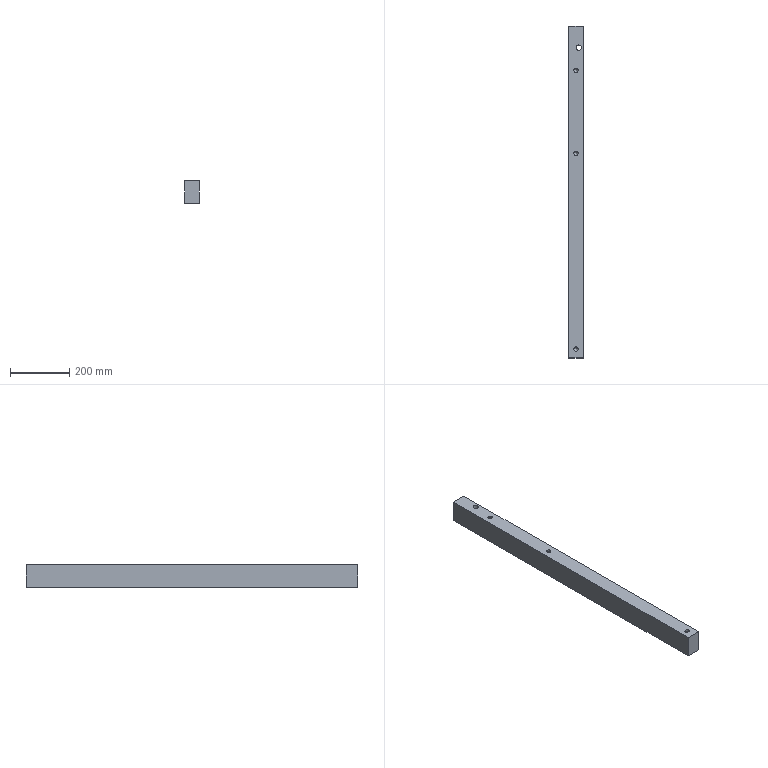Part | NX | features 3 2 | 1 solid | 19 faces | box 50 x 1120 x 75.5 mm | volume 4199138 mm3 | cylinder 7 | plane 6 | cone 6 | commonest cylinder face diameters 14.1 x6 18 x1
STEP:
#1=CARTESIAN_POINT('',(738.05,522.5,256.5));
#2=VERTEX_POINT('',#1);
#3=CARTESIAN_POINT('',(731.,522.5,256.5));
#4=DIRECTION('',(0.,0.,-1.));
#5=DIRECTION('',(1.,0.,0.));
#6=AXIS2_PLACEMENT_3D('',#3,#4,#5);
#7=CIRCLE('',#6,7.05);
#8=EDGE_CURVE('',#2,#2,#7,.T.);
#9=ORIENTED_EDGE('',*,*,#8,.T.);
#10=EDGE_LOOP('',(#9));
#11=FACE_BOUND('',#10,.T.);
#12=CARTESIAN_POINT('',(749.,599.5,256.5));
#13=VERTEX_POINT('',#12);
#14=CARTESIAN_POINT('',(740.,599.5,256.5));
#15=DIRECTION('',(0.,0.,1.));
#16=DIRECTION('',(1.,0.,0.));
#17=AXIS2_PLACEMENT_3D('',#14,#15,#16);
#18=CIRCLE('',#17,9.);
#19=EDGE_CURVE('',#13,#13,#18,.T.);
#20=ORIENTED_EDGE('',*,*,#19,.F.);
#21=EDGE_LOOP('',(#20));
#22=FACE_BOUND('',#21,.T.);
#23=CARTESIAN_POINT('',(756.,-447.5,256.5));
#24=VERTEX_POINT('',#23);
#25=CARTESIAN_POINT('',(706.,-447.5,256.5));
#26=VERTEX_POINT('',#25);
#27=CARTESIAN_POINT('',(283.5,-447.5,256.5));
#28=DIRECTION('',(-1.,0.,0.));
#29=VECTOR('',#28,1000.);
#30=LINE('',#27,#29);
#31=EDGE_CURVE('',#24,#26,#30,.T.);
#32=ORIENTED_EDGE('',*,*,#31,.F.);
#33=CARTESIAN_POINT('',(756.,672.5,256.5));
#34=VERTEX_POINT('',#33);
#35=CARTESIAN_POINT('',(756.,193.,256.5));
#36=DIRECTION('',(0.,-1.,0.));
#37=VECTOR('',#36,1000.);
#38=LINE('',#35,#37);
#39=EDGE_CURVE('',#34,#24,#38,.T.);
#40=ORIENTED_EDGE('',*,*,#39,.F.);
#41=CARTESIAN_POINT('',(706.,672.5,256.5));
#42=VERTEX_POINT('',#41);
#43=CARTESIAN_POINT('',(706.,672.5,256.5));
#44=DIRECTION('',(1.,0.,0.));
#45=VECTOR('',#44,1000.);
#46=LINE('',#43,#45);
#47=EDGE_CURVE('',#42,#34,#46,.T.);
#48=ORIENTED_EDGE('',*,*,#47,.F.);
#49=CARTESIAN_POINT('',(706.,193.,256.5));
#50=DIRECTION('',(0.,1.,0.));
#51=VECTOR('',#50,1000.);
#52=LINE('',#49,#51);
#53=EDGE_CURVE('',#26,#42,#52,.T.);
#54=ORIENTED_EDGE('',*,*,#53,.F.);
#55=EDGE_LOOP('',(#32,#40,#48,#54));
#56=FACE_BOUND('',#55,.T.);
#57=CARTESIAN_POINT('',(738.05,242.5,256.5));
#58=VERTEX_POINT('',#57);
#59=CARTESIAN_POINT('',(731.,242.5,256.5));
#60=DIRECTION('',(0.,0.,-1.));
#61=DIRECTION('',(1.,0.,0.));
#62=AXIS2_PLACEMENT_3D('',#59,#60,#61);
#63=CIRCLE('',#62,7.05);
#64=EDGE_CURVE('',#58,#58,#63,.T.);
#65=ORIENTED_EDGE('',*,*,#64,.T.);
#66=EDGE_LOOP('',(#65));
#67=FACE_BOUND('',#66,.T.);
#68=CARTESIAN_POINT('',(738.05,-417.5,256.5));
#69=VERTEX_POINT('',#68);
#70=CARTESIAN_POINT('',(731.,-417.5,256.5));
#71=DIRECTION('',(0.,0.,-1.));
#72=DIRECTION('',(1.,0.,0.));
#73=AXIS2_PLACEMENT_3D('',#70,#71,#72);
#74=CIRCLE('',#73,7.05);
#75=EDGE_CURVE('',#69,#69,#74,.T.);
#76=ORIENTED_EDGE('',*,*,#75,.T.);
#77=EDGE_LOOP('',(#76));
#78=FACE_BOUND('',#77,.T.);
#79=CARTESIAN_POINT('',(2746.,0.,256.5));
#80=DIRECTION('',(0.,0.,1.));
#81=DIRECTION('',(-1.,0.,0.));
#82=AXIS2_PLACEMENT_3D('',#79,#80,#81);
#83=PLANE('',#82);
#84=ADVANCED_FACE('',(#11,#22,#56,#67,#78),#83,.T.);
#85=CARTESIAN_POINT('',(738.05,522.5,181.));
#86=VERTEX_POINT('',#85);
#87=CARTESIAN_POINT('',(731.,522.5,181.));
#88=DIRECTION('',(0.,0.,1.));
#89=DIRECTION('',(1.,0.,0.));
#90=AXIS2_PLACEMENT_3D('',#87,#88,#89);
#91=CIRCLE('',#90,7.05);
#92=EDGE_CURVE('',#86,#86,#91,.T.);
#93=ORIENTED_EDGE('',*,*,#92,.T.);
#94=EDGE_LOOP('',(#93));
#95=FACE_BOUND('',#94,.T.);
#96=CARTESIAN_POINT('',(731.,599.5,181.));
#97=VERTEX_POINT('',#96);
#98=CARTESIAN_POINT('',(740.,599.5,181.));
#99=DIRECTION('',(0.,0.,-1.));
#100=DIRECTION('',(-1.,0.,0.));
#101=AXIS2_PLACEMENT_3D('',#98,#99,#100);
#102=CIRCLE('',#101,9.);
#103=EDGE_CURVE('',#97,#97,#102,.T.);
#104=ORIENTED_EDGE('',*,*,#103,.F.);
#105=EDGE_LOOP('',(#104));
#106=FACE_BOUND('',#105,.T.);
#107=CARTESIAN_POINT('',(706.,672.5,181.));
#108=VERTEX_POINT('',#107);
#109=CARTESIAN_POINT('',(706.,-447.5,181.));
#110=VERTEX_POINT('',#109);
#111=CARTESIAN_POINT('',(706.,193.,181.));
#112=DIRECTION('',(0.,-1.,0.));
#113=VECTOR('',#112,1000.);
#114=LINE('',#111,#113);
#115=EDGE_CURVE('',#108,#110,#114,.T.);
#116=ORIENTED_EDGE('',*,*,#115,.F.);
#117=CARTESIAN_POINT('',(756.,672.5,181.));
#118=VERTEX_POINT('',#117);
#119=CARTESIAN_POINT('',(1976.,672.5,181.));
#120=DIRECTION('',(1.,0.,0.));
#121=VECTOR('',#120,1000.);
#122=LINE('',#119,#121);
#123=EDGE_CURVE('',#108,#118,#122,.T.);
#124=ORIENTED_EDGE('',*,*,#123,.T.);
#125=CARTESIAN_POINT('',(756.,-447.5,181.));
#126=VERTEX_POINT('',#125);
#127=CARTESIAN_POINT('',(756.,193.,181.));
#128=DIRECTION('',(0.,1.,0.));
#129=VECTOR('',#128,1000.);
#130=LINE('',#127,#129);
#131=EDGE_CURVE('',#126,#118,#130,.T.);
#132=ORIENTED_EDGE('',*,*,#131,.F.);
#133=CARTESIAN_POINT('',(1976.,-447.5,181.));
#134=DIRECTION('',(-1.,0.,0.));
#135=VECTOR('',#134,1000.);
#136=LINE('',#133,#135);
#137=EDGE_CURVE('',#126,#110,#136,.T.);
#138=ORIENTED_EDGE('',*,*,#137,.T.);
#139=EDGE_LOOP('',(#116,#124,#132,#138));
#140=FACE_BOUND('',#139,.T.);
#141=CARTESIAN_POINT('',(738.05,-417.5,181.));
#142=VERTEX_POINT('',#141);
#143=CARTESIAN_POINT('',(731.,-417.5,181.));
#144=DIRECTION('',(0.,0.,1.));
#145=DIRECTION('',(1.,0.,0.));
#146=AXIS2_PLACEMENT_3D('',#143,#144,#145);
#147=CIRCLE('',#146,7.05);
#148=EDGE_CURVE('',#142,#142,#147,.T.);
#149=ORIENTED_EDGE('',*,*,#148,.T.);
#150=EDGE_LOOP('',(#149));
#151=FACE_BOUND('',#150,.T.);
#152=CARTESIAN_POINT('',(738.05,242.5,181.));
#153=VERTEX_POINT('',#152);
#154=CARTESIAN_POINT('',(731.,242.5,181.));
#155=DIRECTION('',(0.,0.,1.));
#156=DIRECTION('',(1.,0.,0.));
#157=AXIS2_PLACEMENT_3D('',#154,#155,#156);
#158=CIRCLE('',#157,7.05);
#159=EDGE_CURVE('',#153,#153,#158,.T.);
#160=ORIENTED_EDGE('',*,*,#159,.T.);
#161=EDGE_LOOP('',(#160));
#162=FACE_BOUND('',#161,.T.);
#163=CARTESIAN_POINT('',(1976.,193.,181.));
#164=DIRECTION('',(0.,0.,-1.));
#165=DIRECTION('',(-1.,0.,0.));
#166=AXIS2_PLACEMENT_3D('',#163,#164,#165);
#167=PLANE('',#166);
#168=ADVANCED_FACE('',(#95,#106,#140,#151,#162),#167,.T.);
#169=CARTESIAN_POINT('',(706.,-447.5,-1.5));
#170=DIRECTION('',(0.,0.,1.));
#171=VECTOR('',#170,1000.);
#172=LINE('',#169,#171);
#173=EDGE_CURVE('',#110,#26,#172,.T.);
#174=ORIENTED_EDGE('',*,*,#173,.T.);
#175=ORIENTED_EDGE('',*,*,#53,.T.);
#176=CARTESIAN_POINT('',(706.,672.5,-1.5));
#177=DIRECTION('',(0.,0.,-1.));
#178=VECTOR('',#177,1000.);
#179=LINE('',#176,#178);
#180=EDGE_CURVE('',#42,#108,#179,.T.);
#181=ORIENTED_EDGE('',*,*,#180,.T.);
#182=ORIENTED_EDGE('',*,*,#115,.T.);
#183=EDGE_LOOP('',(#174,#175,#181,#182));
#184=FACE_BOUND('',#183,.T.);
#185=CARTESIAN_POINT('',(706.,193.,-1.5));
#186=DIRECTION('',(-1.,0.,0.));
#187=DIRECTION('',(0.,0.,-1.));
#188=AXIS2_PLACEMENT_3D('',#185,#186,#187);
#189=PLANE('',#188);
#190=ADVANCED_FACE('',(#184),#189,.T.);
#191=CARTESIAN_POINT('',(756.,672.5,-1.5));
#192=DIRECTION('',(0.,0.,1.));
#193=VECTOR('',#192,1000.);
#194=LINE('',#191,#193);
#195=EDGE_CURVE('',#118,#34,#194,.T.);
#196=ORIENTED_EDGE('',*,*,#195,.T.);
#197=ORIENTED_EDGE('',*,*,#39,.T.);
#198=CARTESIAN_POINT('',(756.,-447.5,-1.5));
#199=DIRECTION('',(0.,0.,-1.));
#200=VECTOR('',#199,1000.);
#201=LINE('',#198,#200);
#202=EDGE_CURVE('',#24,#126,#201,.T.);
#203=ORIENTED_EDGE('',*,*,#202,.T.);
#204=ORIENTED_EDGE('',*,*,#131,.T.);
#205=EDGE_LOOP('',(#196,#197,#203,#204));
#206=FACE_BOUND('',#205,.T.);
#207=CARTESIAN_POINT('',(756.,193.,-1.5));
#208=DIRECTION('',(1.,0.,0.));
#209=DIRECTION('',(0.,0.,1.));
#210=AXIS2_PLACEMENT_3D('',#207,#208,#209);
#211=PLANE('',#210);
#212=ADVANCED_FACE('',(#206),#211,.T.);
#213=ORIENTED_EDGE('',*,*,#202,.F.);
#214=ORIENTED_EDGE('',*,*,#31,.T.);
#215=ORIENTED_EDGE('',*,*,#173,.F.);
#216=ORIENTED_EDGE('',*,*,#137,.F.);
#217=EDGE_LOOP('',(#213,#214,#215,#216));
#218=FACE_BOUND('',#217,.T.);
#219=CARTESIAN_POINT('',(283.5,-447.5,-103.));
#220=DIRECTION('',(0.,1.,0.));
#221=DIRECTION('',(1.,0.,0.));
#222=AXIS2_PLACEMENT_3D('',#219,#220,#221);
#223=PLANE('',#222);
#224=ADVANCED_FACE('',(#218),#223,.F.);
#225=ORIENTED_EDGE('',*,*,#180,.F.);
#226=ORIENTED_EDGE('',*,*,#47,.T.);
#227=ORIENTED_EDGE('',*,*,#195,.F.);
#228=ORIENTED_EDGE('',*,*,#123,.F.);
#229=EDGE_LOOP('',(#225,#226,#227,#228));
#230=FACE_BOUND('',#229,.T.);
#231=CARTESIAN_POINT('',(706.,672.5,231.5));
#232=DIRECTION('',(0.,1.,0.));
#233=DIRECTION('',(0.,0.,-1.));
#234=AXIS2_PLACEMENT_3D('',#231,#232,#233);
#235=PLANE('',#234);
#236=ADVANCED_FACE('',(#230),#235,.T.);
#237=ORIENTED_EDGE('',*,*,#19,.T.);
#238=EDGE_LOOP('',(#237));
#239=FACE_BOUND('',#238,.T.);
#240=ORIENTED_EDGE('',*,*,#103,.T.);
#241=EDGE_LOOP('',(#240));
#242=FACE_BOUND('',#241,.T.);
#243=CARTESIAN_POINT('',(740.,599.5,-306.5));
#244=DIRECTION('',(0.,0.,1.));
#245=DIRECTION('',(-1.,0.,0.));
#246=AXIS2_PLACEMENT_3D('',#243,#244,#245);
#247=CYLINDRICAL_SURFACE('',#246,9.);
#248=ADVANCED_FACE('',(#239,#242),#247,.F.);
#249=CARTESIAN_POINT('',(738.05,-417.5,188.95));
#250=VERTEX_POINT('',#249);
#251=CARTESIAN_POINT('',(731.,-417.5,188.95));
#252=DIRECTION('',(0.,0.,1.));
#253=DIRECTION('',(1.,0.,0.));
#254=AXIS2_PLACEMENT_3D('',#251,#252,#253);
#255=CIRCLE('',#254,7.05);
#256=EDGE_CURVE('',#250,#250,#255,.T.);
#257=ORIENTED_EDGE('',*,*,#256,.T.);
#258=EDGE_LOOP('',(#257));
#259=FACE_BOUND('',#258,.T.);
#260=ORIENTED_EDGE('',*,*,#148,.F.);
#261=EDGE_LOOP('',(#260));
#262=FACE_BOUND('',#261,.T.);
#263=CARTESIAN_POINT('',(731.,-417.5,181.));
#264=DIRECTION('',(0.,0.,1.));
#265=DIRECTION('',(-1.,0.,0.));
#266=AXIS2_PLACEMENT_3D('',#263,#264,#265);
#267=CYLINDRICAL_SURFACE('',#266,7.05);
#268=ADVANCED_FACE('',(#259,#262),#267,.F.);
#269=CARTESIAN_POINT('',(731.,-417.5,196.));
#270=VERTEX_POINT('',#269);
#271=VERTEX_LOOP('',#270);
#272=FACE_BOUND('',#271,.T.);
#273=ORIENTED_EDGE('',*,*,#256,.F.);
#274=EDGE_LOOP('',(#273));
#275=FACE_BOUND('',#274,.T.);
#276=CARTESIAN_POINT('',(731.,-417.5,188.95));
#277=DIRECTION('',(0.,0.,-1.));
#278=DIRECTION('',(1.,0.,0.));
#279=AXIS2_PLACEMENT_3D('',#276,#277,#278);
#280=CONICAL_SURFACE('',#279,7.05,0.7854);
#281=ADVANCED_FACE('',(#272,#275),#280,.F.);
#282=CARTESIAN_POINT('',(738.05,522.5,188.95));
#283=VERTEX_POINT('',#282);
#284=CARTESIAN_POINT('',(731.,522.5,188.95));
#285=DIRECTION('',(0.,0.,1.));
#286=DIRECTION('',(1.,0.,0.));
#287=AXIS2_PLACEMENT_3D('',#284,#285,#286);
#288=CIRCLE('',#287,7.05);
#289=EDGE_CURVE('',#283,#283,#288,.T.);
#290=ORIENTED_EDGE('',*,*,#289,.T.);
#291=EDGE_LOOP('',(#290));
#292=FACE_BOUND('',#291,.T.);
#293=ORIENTED_EDGE('',*,*,#92,.F.);
#294=EDGE_LOOP('',(#293));
#295=FACE_BOUND('',#294,.T.);
#296=CARTESIAN_POINT('',(731.,522.5,181.));
#297=DIRECTION('',(0.,0.,1.));
#298=DIRECTION('',(-1.,0.,0.));
#299=AXIS2_PLACEMENT_3D('',#296,#297,#298);
#300=CYLINDRICAL_SURFACE('',#299,7.05);
#301=ADVANCED_FACE('',(#292,#295),#300,.F.);
#302=CARTESIAN_POINT('',(731.,522.5,196.));
#303=VERTEX_POINT('',#302);
#304=VERTEX_LOOP('',#303);
#305=FACE_BOUND('',#304,.T.);
#306=ORIENTED_EDGE('',*,*,#289,.F.);
#307=EDGE_LOOP('',(#306));
#308=FACE_BOUND('',#307,.T.);
#309=CARTESIAN_POINT('',(731.,522.5,188.95));
#310=DIRECTION('',(0.,0.,-1.));
#311=DIRECTION('',(1.,0.,0.));
#312=AXIS2_PLACEMENT_3D('',#309,#310,#311);
#313=CONICAL_SURFACE('',#312,7.05,0.7854);
#314=ADVANCED_FACE('',(#305,#308),#313,.F.);
#315=CARTESIAN_POINT('',(738.05,242.5,188.95));
#316=VERTEX_POINT('',#315);
#317=CARTESIAN_POINT('',(731.,242.5,188.95));
#318=DIRECTION('',(0.,0.,1.));
#319=DIRECTION('',(1.,0.,0.));
#320=AXIS2_PLACEMENT_3D('',#317,#318,#319);
#321=CIRCLE('',#320,7.05);
#322=EDGE_CURVE('',#316,#316,#321,.T.);
#323=ORIENTED_EDGE('',*,*,#322,.T.);
#324=EDGE_LOOP('',(#323));
#325=FACE_BOUND('',#324,.T.);
#326=ORIENTED_EDGE('',*,*,#159,.F.);
#327=EDGE_LOOP('',(#326));
#328=FACE_BOUND('',#327,.T.);
#329=CARTESIAN_POINT('',(731.,242.5,181.));
#330=DIRECTION('',(0.,0.,1.));
#331=DIRECTION('',(-1.,0.,0.));
#332=AXIS2_PLACEMENT_3D('',#329,#330,#331);
#333=CYLINDRICAL_SURFACE('',#332,7.05);
#334=ADVANCED_FACE('',(#325,#328),#333,.F.);
#335=CARTESIAN_POINT('',(731.,242.5,196.));
#336=VERTEX_POINT('',#335);
#337=VERTEX_LOOP('',#336);
#338=FACE_BOUND('',#337,.T.);
#339=ORIENTED_EDGE('',*,*,#322,.F.);
#340=EDGE_LOOP('',(#339));
#341=FACE_BOUND('',#340,.T.);
#342=CARTESIAN_POINT('',(731.,242.5,188.95));
#343=DIRECTION('',(0.,0.,-1.));
#344=DIRECTION('',(1.,0.,0.));
#345=AXIS2_PLACEMENT_3D('',#342,#343,#344);
#346=CONICAL_SURFACE('',#345,7.05,0.7854);
#347=ADVANCED_FACE('',(#338,#341),#346,.F.);
#348=CARTESIAN_POINT('',(723.95,242.5,248.55));
#349=VERTEX_POINT('',#348);
#350=CARTESIAN_POINT('',(731.,242.5,248.55));
#351=DIRECTION('',(0.,0.,-1.));
#352=DIRECTION('',(-1.,0.,0.));
#353=AXIS2_PLACEMENT_3D('',#350,#351,#352);
#354=CIRCLE('',#353,7.05);
#355=EDGE_CURVE('',#349,#349,#354,.T.);
#356=ORIENTED_EDGE('',*,*,#355,.T.);
#357=EDGE_LOOP('',(#356));
#358=FACE_BOUND('',#357,.T.);
#359=ORIENTED_EDGE('',*,*,#64,.F.);
#360=EDGE_LOOP('',(#359));
#361=FACE_BOUND('',#360,.T.);
#362=CARTESIAN_POINT('',(731.,242.5,256.5));
#363=DIRECTION('',(0.,0.,-1.));
#364=DIRECTION('',(-1.,0.,0.));
#365=AXIS2_PLACEMENT_3D('',#362,#363,#364);
#366=CYLINDRICAL_SURFACE('',#365,7.05);
#367=ADVANCED_FACE('',(#358,#361),#366,.F.);
#368=CARTESIAN_POINT('',(731.,242.5,241.5));
#369=VERTEX_POINT('',#368);
#370=VERTEX_LOOP('',#369);
#371=FACE_BOUND('',#370,.T.);
#372=ORIENTED_EDGE('',*,*,#355,.F.);
#373=EDGE_LOOP('',(#372));
#374=FACE_BOUND('',#373,.T.);
#375=CARTESIAN_POINT('',(731.,242.5,248.55));
#376=DIRECTION('',(0.,0.,1.));
#377=DIRECTION('',(-1.,0.,0.));
#378=AXIS2_PLACEMENT_3D('',#375,#376,#377);
#379=CONICAL_SURFACE('',#378,7.05,0.7854);
#380=ADVANCED_FACE('',(#371,#374),#379,.F.);
#381=CARTESIAN_POINT('',(723.95,522.5,248.55));
#382=VERTEX_POINT('',#381);
#383=CARTESIAN_POINT('',(731.,522.5,248.55));
#384=DIRECTION('',(0.,0.,-1.));
#385=DIRECTION('',(-1.,0.,0.));
#386=AXIS2_PLACEMENT_3D('',#383,#384,#385);
#387=CIRCLE('',#386,7.05);
#388=EDGE_CURVE('',#382,#382,#387,.T.);
#389=ORIENTED_EDGE('',*,*,#388,.T.);
#390=EDGE_LOOP('',(#389));
#391=FACE_BOUND('',#390,.T.);
#392=ORIENTED_EDGE('',*,*,#8,.F.);
#393=EDGE_LOOP('',(#392));
#394=FACE_BOUND('',#393,.T.);
#395=CARTESIAN_POINT('',(731.,522.5,256.5));
#396=DIRECTION('',(0.,0.,-1.));
#397=DIRECTION('',(-1.,0.,0.));
#398=AXIS2_PLACEMENT_3D('',#395,#396,#397);
#399=CYLINDRICAL_SURFACE('',#398,7.05);
#400=ADVANCED_FACE('',(#391,#394),#399,.F.);
#401=CARTESIAN_POINT('',(731.,522.5,241.5));
#402=VERTEX_POINT('',#401);
#403=VERTEX_LOOP('',#402);
#404=FACE_BOUND('',#403,.T.);
#405=ORIENTED_EDGE('',*,*,#388,.F.);
#406=EDGE_LOOP('',(#405));
#407=FACE_BOUND('',#406,.T.);
#408=CARTESIAN_POINT('',(731.,522.5,248.55));
#409=DIRECTION('',(0.,0.,1.));
#410=DIRECTION('',(-1.,0.,0.));
#411=AXIS2_PLACEMENT_3D('',#408,#409,#410);
#412=CONICAL_SURFACE('',#411,7.05,0.7854);
#413=ADVANCED_FACE('',(#404,#407),#412,.F.);
#414=CARTESIAN_POINT('',(723.95,-417.5,248.55));
#415=VERTEX_POINT('',#414);
#416=CARTESIAN_POINT('',(731.,-417.5,248.55));
#417=DIRECTION('',(0.,0.,-1.));
#418=DIRECTION('',(-1.,0.,0.));
#419=AXIS2_PLACEMENT_3D('',#416,#417,#418);
#420=CIRCLE('',#419,7.05);
#421=EDGE_CURVE('',#415,#415,#420,.T.);
#422=ORIENTED_EDGE('',*,*,#421,.T.);
#423=EDGE_LOOP('',(#422));
#424=FACE_BOUND('',#423,.T.);
#425=ORIENTED_EDGE('',*,*,#75,.F.);
#426=EDGE_LOOP('',(#425));
#427=FACE_BOUND('',#426,.T.);
#428=CARTESIAN_POINT('',(731.,-417.5,256.5));
#429=DIRECTION('',(0.,0.,-1.));
#430=DIRECTION('',(-1.,0.,0.));
#431=AXIS2_PLACEMENT_3D('',#428,#429,#430);
#432=CYLINDRICAL_SURFACE('',#431,7.05);
#433=ADVANCED_FACE('',(#424,#427),#432,.F.);
#434=CARTESIAN_POINT('',(731.,-417.5,241.5));
#435=VERTEX_POINT('',#434);
#436=VERTEX_LOOP('',#435);
#437=FACE_BOUND('',#436,.T.);
#438=ORIENTED_EDGE('',*,*,#421,.F.);
#439=EDGE_LOOP('',(#438));
#440=FACE_BOUND('',#439,.T.);
#441=CARTESIAN_POINT('',(731.,-417.5,248.55));
#442=DIRECTION('',(0.,0.,1.));
#443=DIRECTION('',(-1.,0.,0.));
#444=AXIS2_PLACEMENT_3D('',#441,#442,#443);
#445=CONICAL_SURFACE('',#444,7.05,0.7854);
#446=ADVANCED_FACE('',(#437,#440),#445,.F.);
#447=CLOSED_SHELL('',(#84,#168,#190,#212,#224,#236,#248,#268,#281,#301,#314,#334,#347,#367,#380,#400,#413,#433,#446));
#448=MANIFOLD_SOLID_BREP('',#447);
#449=(LENGTH_UNIT()NAMED_UNIT(*)SI_UNIT(.MILLI.,.METRE.));
#450=UNCERTAINTY_MEASURE_WITH_UNIT(LENGTH_MEASURE(0.00001),#449,'','');
#451=(NAMED_UNIT(*)PLANE_ANGLE_UNIT()SI_UNIT($,.RADIAN.));
#452=(NAMED_UNIT(*)SI_UNIT($,.STERADIAN.)SOLID_ANGLE_UNIT());
#453=(GEOMETRIC_REPRESENTATION_CONTEXT(3)GLOBAL_UNCERTAINTY_ASSIGNED_CONTEXT((#450))GLOBAL_UNIT_ASSIGNED_CONTEXT((#449,#451,#452))REPRESENTATION_CONTEXT('',''));
#454=ADVANCED_BREP_SHAPE_REPRESENTATION('',(#448),#453);